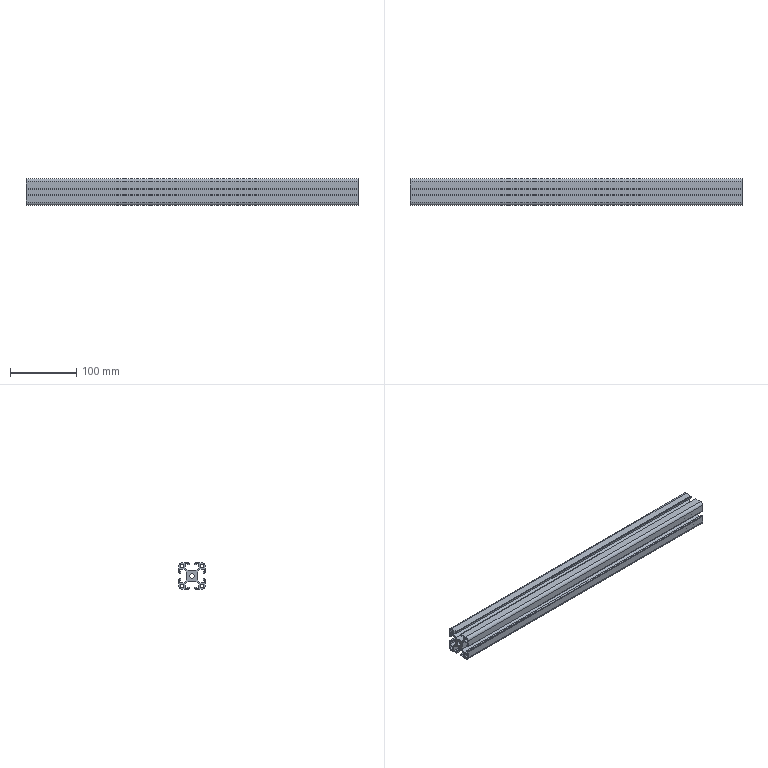Part | SolidWorks | features WeldMemberFeat 1, WeldmentFeature 1 | 1 solid | 104 faces | box 500 x 40 x 40 mm | volume 288273 mm3 | plane 94 | cylinder 10 | commonest cylinder face diameters 5 x4 9 x4 6.8 x2